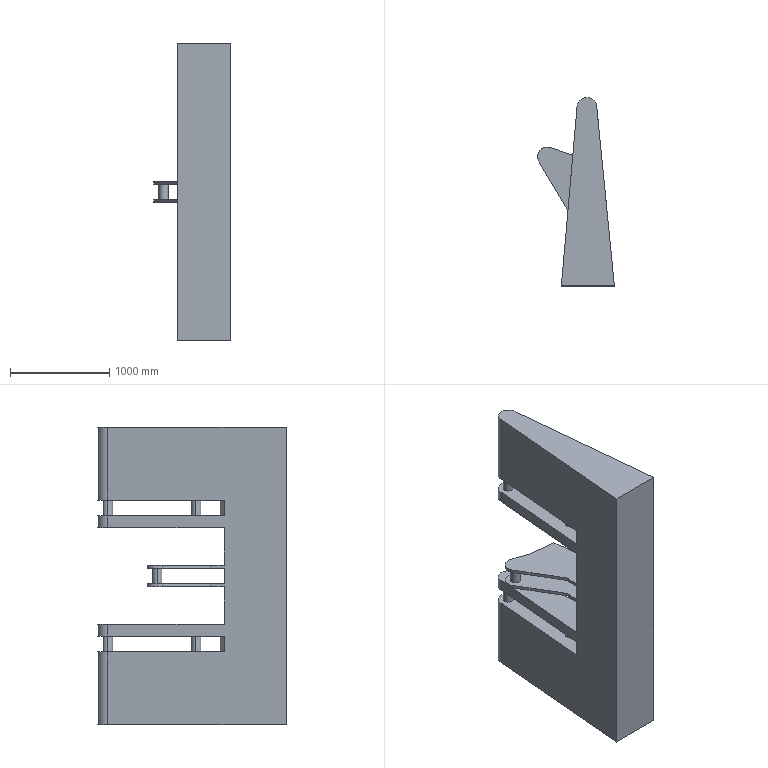Part | SolidWorks | features ICE 8, MirrorPattern 4, Extrusion 1 | 1 solid | 43 faces | box 773.621 x 1900 x 3000 mm | volume 1564577598 mm3 | plane 26 | cylinder 17 | commonest cylinder face diameters 100 x10 200 x7
STEP:
#1=CARTESIAN_POINT('',(534.418,439.01,-2105.5));
#2=VERTEX_POINT('',#1);
#3=CARTESIAN_POINT('',(434.418,439.01,-2105.5));
#4=VERTEX_POINT('',#3);
#5=CARTESIAN_POINT('',(484.418,439.01,-2105.5));
#6=DIRECTION('',(0.,0.,1.));
#7=DIRECTION('',(0.,1.,0.));
#8=AXIS2_PLACEMENT_3D('',#5,#6,#7);
#9=CIRCLE('',#8,50.);
#10=EDGE_CURVE('',#2,#4,#9,.T.);
#11=ORIENTED_EDGE('',*,*,#10,.F.);
#12=CARTESIAN_POINT('',(534.418,439.01,-2265.5));
#13=VERTEX_POINT('',#12);
#14=CARTESIAN_POINT('',(534.418,439.01,-873.079));
#15=DIRECTION('',(0.,0.,-1.));
#16=VECTOR('',#15,1000.);
#17=LINE('',#14,#16);
#18=EDGE_CURVE('',#2,#13,#17,.T.);
#19=ORIENTED_EDGE('',*,*,#18,.T.);
#20=CARTESIAN_POINT('',(434.418,439.01,-2265.5));
#21=VERTEX_POINT('',#20);
#22=CARTESIAN_POINT('',(484.418,439.01,-2265.5));
#23=DIRECTION('',(0.,0.,-1.));
#24=DIRECTION('',(1.,0.,0.));
#25=AXIS2_PLACEMENT_3D('',#22,#23,#24);
#26=CIRCLE('',#25,50.);
#27=EDGE_CURVE('',#21,#13,#26,.T.);
#28=ORIENTED_EDGE('',*,*,#27,.F.);
#29=CARTESIAN_POINT('',(434.418,439.01,-873.079));
#30=DIRECTION('',(0.,0.,-1.));
#31=VECTOR('',#30,1000.);
#32=LINE('',#29,#31);
#33=EDGE_CURVE('',#4,#21,#32,.T.);
#34=ORIENTED_EDGE('',*,*,#33,.F.);
#35=EDGE_LOOP('',(#11,#19,#28,#34));
#36=FACE_OUTER_BOUND('',#35,.T.);
#37=CARTESIAN_POINT('',(484.418,439.01,-873.079));
#38=DIRECTION('',(0.,0.,-1.));
#39=DIRECTION('',(-1.,0.,0.));
#40=AXIS2_PLACEMENT_3D('',#37,#38,#39);
#41=CYLINDRICAL_SURFACE('',#40,50.);
#42=ADVANCED_FACE('',(#36),#41,.T.);
#43=CARTESIAN_POINT('',(434.418,439.01,-894.5));
#44=VERTEX_POINT('',#43);
#45=CARTESIAN_POINT('',(534.418,439.01,-894.5));
#46=VERTEX_POINT('',#45);
#47=CARTESIAN_POINT('',(484.418,439.01,-894.5));
#48=DIRECTION('',(0.,0.,-1.));
#49=DIRECTION('',(0.,1.,0.));
#50=AXIS2_PLACEMENT_3D('',#47,#48,#49);
#51=CIRCLE('',#50,50.);
#52=EDGE_CURVE('',#44,#46,#51,.T.);
#53=ORIENTED_EDGE('',*,*,#52,.F.);
#54=CARTESIAN_POINT('',(434.418,439.01,-734.5));
#55=VERTEX_POINT('',#54);
#56=CARTESIAN_POINT('',(434.418,439.01,-1155.921));
#57=DIRECTION('',(0.,0.,1.));
#58=VECTOR('',#57,1000.);
#59=LINE('',#56,#58);
#60=EDGE_CURVE('',#44,#55,#59,.T.);
#61=ORIENTED_EDGE('',*,*,#60,.T.);
#62=CARTESIAN_POINT('',(534.418,439.01,-734.5));
#63=VERTEX_POINT('',#62);
#64=CARTESIAN_POINT('',(484.418,439.01,-734.5));
#65=DIRECTION('',(0.,0.,1.));
#66=DIRECTION('',(1.,0.,0.));
#67=AXIS2_PLACEMENT_3D('',#64,#65,#66);
#68=CIRCLE('',#67,50.);
#69=EDGE_CURVE('',#63,#55,#68,.T.);
#70=ORIENTED_EDGE('',*,*,#69,.F.);
#71=CARTESIAN_POINT('',(534.418,439.01,-1155.921));
#72=DIRECTION('',(0.,0.,1.));
#73=VECTOR('',#72,1000.);
#74=LINE('',#71,#73);
#75=EDGE_CURVE('',#46,#63,#74,.T.);
#76=ORIENTED_EDGE('',*,*,#75,.F.);
#77=EDGE_LOOP('',(#53,#61,#70,#76));
#78=FACE_OUTER_BOUND('',#77,.T.);
#79=CARTESIAN_POINT('',(484.418,439.01,-1155.921));
#80=DIRECTION('',(0.,0.,1.));
#81=DIRECTION('',(1.,0.,0.));
#82=AXIS2_PLACEMENT_3D('',#79,#80,#81);
#83=CYLINDRICAL_SURFACE('',#82,50.);
#84=ADVANCED_FACE('',(#78),#83,.T.);
#85=CARTESIAN_POINT('',(137.752,831.385,-1580.));
#86=VERTEX_POINT('',#85);
#87=CARTESIAN_POINT('',(37.752,831.385,-1580.));
#88=VERTEX_POINT('',#87);
#89=CARTESIAN_POINT('',(87.752,831.385,-1580.));
#90=DIRECTION('',(0.,0.,1.));
#91=DIRECTION('',(1.,0.,0.));
#92=AXIS2_PLACEMENT_3D('',#89,#90,#91);
#93=CIRCLE('',#92,50.);
#94=EDGE_CURVE('',#86,#88,#93,.T.);
#95=ORIENTED_EDGE('',*,*,#94,.T.);
#96=CARTESIAN_POINT('',(37.752,831.385,-1420.));
#97=VERTEX_POINT('',#96);
#98=CARTESIAN_POINT('',(37.752,831.385,-1751.421));
#99=DIRECTION('',(0.,0.,1.));
#100=VECTOR('',#99,1000.);
#101=LINE('',#98,#100);
#102=EDGE_CURVE('',#88,#97,#101,.T.);
#103=ORIENTED_EDGE('',*,*,#102,.T.);
#104=CARTESIAN_POINT('',(137.752,831.385,-1420.));
#105=VERTEX_POINT('',#104);
#106=CARTESIAN_POINT('',(87.752,831.385,-1420.));
#107=DIRECTION('',(0.,0.,-1.));
#108=DIRECTION('',(1.,0.,0.));
#109=AXIS2_PLACEMENT_3D('',#106,#107,#108);
#110=CIRCLE('',#109,50.);
#111=EDGE_CURVE('',#97,#105,#110,.T.);
#112=ORIENTED_EDGE('',*,*,#111,.T.);
#113=CARTESIAN_POINT('',(137.752,831.385,-1751.421));
#114=DIRECTION('',(0.,0.,1.));
#115=VECTOR('',#114,1000.);
#116=LINE('',#113,#115);
#117=EDGE_CURVE('',#86,#105,#116,.T.);
#118=ORIENTED_EDGE('',*,*,#117,.F.);
#119=EDGE_LOOP('',(#95,#103,#112,#118));
#120=FACE_OUTER_BOUND('',#119,.T.);
#121=CARTESIAN_POINT('',(87.752,831.385,-1751.421));
#122=DIRECTION('',(0.,0.,1.));
#123=DIRECTION('',(1.,0.,0.));
#124=AXIS2_PLACEMENT_3D('',#121,#122,#123);
#125=CYLINDRICAL_SURFACE('',#124,50.);
#126=ADVANCED_FACE('',(#120),#125,.T.);
#127=CARTESIAN_POINT('',(434.418,1329.01,-894.5));
#128=VERTEX_POINT('',#127);
#129=CARTESIAN_POINT('',(534.418,1329.01,-894.5));
#130=VERTEX_POINT('',#129);
#131=CARTESIAN_POINT('',(484.418,1329.01,-894.5));
#132=DIRECTION('',(0.,0.,-1.));
#133=DIRECTION('',(0.,1.,0.));
#134=AXIS2_PLACEMENT_3D('',#131,#132,#133);
#135=CIRCLE('',#134,50.);
#136=EDGE_CURVE('',#128,#130,#135,.T.);
#137=ORIENTED_EDGE('',*,*,#136,.F.);
#138=CARTESIAN_POINT('',(434.418,1329.01,-734.5));
#139=VERTEX_POINT('',#138);
#140=CARTESIAN_POINT('',(434.418,1329.01,-3000.));
#141=DIRECTION('',(0.,0.,1.));
#142=VECTOR('',#141,1000.);
#143=LINE('',#140,#142);
#144=EDGE_CURVE('',#128,#139,#143,.T.);
#145=ORIENTED_EDGE('',*,*,#144,.T.);
#146=CARTESIAN_POINT('',(534.418,1329.01,-734.5));
#147=VERTEX_POINT('',#146);
#148=CARTESIAN_POINT('',(484.418,1329.01,-734.5));
#149=DIRECTION('',(0.,0.,1.));
#150=DIRECTION('',(1.,0.,0.));
#151=AXIS2_PLACEMENT_3D('',#148,#149,#150);
#152=CIRCLE('',#151,50.);
#153=EDGE_CURVE('',#147,#139,#152,.T.);
#154=ORIENTED_EDGE('',*,*,#153,.F.);
#155=CARTESIAN_POINT('',(534.418,1329.01,-3000.));
#156=DIRECTION('',(0.,0.,1.));
#157=VECTOR('',#156,1000.);
#158=LINE('',#155,#157);
#159=EDGE_CURVE('',#130,#147,#158,.T.);
#160=ORIENTED_EDGE('',*,*,#159,.F.);
#161=EDGE_LOOP('',(#137,#145,#154,#160));
#162=FACE_OUTER_BOUND('',#161,.T.);
#163=CARTESIAN_POINT('',(484.418,1329.01,-3000.));
#164=DIRECTION('',(0.,0.,1.));
#165=DIRECTION('',(1.,0.,0.));
#166=AXIS2_PLACEMENT_3D('',#163,#164,#165);
#167=CYLINDRICAL_SURFACE('',#166,50.);
#168=ADVANCED_FACE('',(#162),#167,.T.);
#169=CARTESIAN_POINT('',(534.418,1329.01,-2265.5));
#170=VERTEX_POINT('',#169);
#171=CARTESIAN_POINT('',(434.418,1329.01,-2265.5));
#172=VERTEX_POINT('',#171);
#173=CARTESIAN_POINT('',(484.418,1329.01,-2265.5));
#174=DIRECTION('',(0.,0.,1.));
#175=DIRECTION('',(1.,0.,0.));
#176=AXIS2_PLACEMENT_3D('',#173,#174,#175);
#177=CIRCLE('',#176,50.);
#178=EDGE_CURVE('',#170,#172,#177,.T.);
#179=ORIENTED_EDGE('',*,*,#178,.T.);
#180=CARTESIAN_POINT('',(434.418,1329.01,-2105.5));
#181=VERTEX_POINT('',#180);
#182=CARTESIAN_POINT('',(434.418,1329.01,-3000.));
#183=DIRECTION('',(0.,0.,1.));
#184=VECTOR('',#183,1000.);
#185=LINE('',#182,#184);
#186=EDGE_CURVE('',#172,#181,#185,.T.);
#187=ORIENTED_EDGE('',*,*,#186,.T.);
#188=CARTESIAN_POINT('',(534.418,1329.01,-2105.5));
#189=VERTEX_POINT('',#188);
#190=CARTESIAN_POINT('',(484.418,1329.01,-2105.5));
#191=DIRECTION('',(0.,0.,-1.));
#192=DIRECTION('',(0.,1.,0.));
#193=AXIS2_PLACEMENT_3D('',#190,#191,#192);
#194=CIRCLE('',#193,50.);
#195=EDGE_CURVE('',#181,#189,#194,.T.);
#196=ORIENTED_EDGE('',*,*,#195,.T.);
#197=CARTESIAN_POINT('',(534.418,1329.01,-3000.));
#198=DIRECTION('',(0.,0.,1.));
#199=VECTOR('',#198,1000.);
#200=LINE('',#197,#199);
#201=EDGE_CURVE('',#170,#189,#200,.T.);
#202=ORIENTED_EDGE('',*,*,#201,.F.);
#203=EDGE_LOOP('',(#179,#187,#196,#202));
#204=FACE_OUTER_BOUND('',#203,.T.);
#205=CARTESIAN_POINT('',(484.418,1329.01,-3000.));
#206=DIRECTION('',(0.,0.,1.));
#207=DIRECTION('',(1.,0.,0.));
#208=AXIS2_PLACEMENT_3D('',#205,#206,#207);
#209=CYLINDRICAL_SURFACE('',#208,50.);
#210=ADVANCED_FACE('',(#204),#209,.T.);
#211=CARTESIAN_POINT('',(-12.248,831.385,-1580.));
#212=VERTEX_POINT('',#211);
#213=CARTESIAN_POINT('',(1.855,780.182,-1580.));
#214=VERTEX_POINT('',#213);
#215=CARTESIAN_POINT('',(87.752,831.385,-1580.));
#216=DIRECTION('',(0.,0.,1.));
#217=DIRECTION('',(1.,0.,0.));
#218=AXIS2_PLACEMENT_3D('',#215,#216,#217);
#219=CIRCLE('',#218,100.);
#220=EDGE_CURVE('',#212,#214,#219,.T.);
#221=ORIENTED_EDGE('',*,*,#220,.F.);
#222=CARTESIAN_POINT('',(-12.248,831.385,-1610.));
#223=VERTEX_POINT('',#222);
#224=CARTESIAN_POINT('',(-12.248,831.385,-1580.));
#225=DIRECTION('',(0.,0.,-1.));
#226=VECTOR('',#225,1000.);
#227=LINE('',#224,#226);
#228=EDGE_CURVE('',#212,#223,#227,.T.);
#229=ORIENTED_EDGE('',*,*,#228,.T.);
#230=CARTESIAN_POINT('',(1.855,780.182,-1610.));
#231=VERTEX_POINT('',#230);
#232=CARTESIAN_POINT('',(87.752,831.385,-1610.));
#233=DIRECTION('',(0.,0.,1.));
#234=DIRECTION('',(1.,0.,0.));
#235=AXIS2_PLACEMENT_3D('',#232,#233,#234);
#236=CIRCLE('',#235,100.);
#237=EDGE_CURVE('',#223,#231,#236,.T.);
#238=ORIENTED_EDGE('',*,*,#237,.T.);
#239=CARTESIAN_POINT('',(1.855,780.182,-1580.));
#240=DIRECTION('',(0.,0.,-1.));
#241=VECTOR('',#240,1000.);
#242=LINE('',#239,#241);
#243=EDGE_CURVE('',#214,#231,#242,.T.);
#244=ORIENTED_EDGE('',*,*,#243,.F.);
#245=EDGE_LOOP('',(#221,#229,#238,#244));
#246=FACE_OUTER_BOUND('',#245,.T.);
#247=CARTESIAN_POINT('',(87.752,831.385,-1580.));
#248=DIRECTION('',(0.,0.,-1.));
#249=DIRECTION('',(-1.,0.,0.));
#250=AXIS2_PLACEMENT_3D('',#247,#248,#249);
#251=CYLINDRICAL_SURFACE('',#250,100.);
#252=ADVANCED_FACE('',(#246),#251,.T.);
#253=CARTESIAN_POINT('',(342.529,850.219,-1390.));
#254=VERTEX_POINT('',#253);
#255=CARTESIAN_POINT('',(633.994,824.719,-1390.));
#256=VERTEX_POINT('',#255);
#257=CARTESIAN_POINT('',(76.421,873.5,-1390.));
#258=DIRECTION('',(0.9962,-0.08716,0.));
#259=VECTOR('',#258,1000.);
#260=LINE('',#257,#259);
#261=EDGE_CURVE('',#254,#256,#260,.T.);
#262=ORIENTED_EDGE('',*,*,#261,.F.);
#263=CARTESIAN_POINT('',(120.005,926.041,-1390.));
#264=VERTEX_POINT('',#263);
#265=CARTESIAN_POINT('',(295.197,866.347,-1390.));
#266=DIRECTION('',(0.9466,-0.3225,0.));
#267=VECTOR('',#266,1000.);
#268=LINE('',#265,#267);
#269=EDGE_CURVE('',#264,#254,#268,.T.);
#270=ORIENTED_EDGE('',*,*,#269,.F.);
#271=CARTESIAN_POINT('',(1.855,780.182,-1390.));
#272=VERTEX_POINT('',#271);
#273=CARTESIAN_POINT('',(87.752,831.385,-1390.));
#274=DIRECTION('',(0.,0.,1.));
#275=DIRECTION('',(1.,0.,0.));
#276=AXIS2_PLACEMENT_3D('',#273,#274,#275);
#277=CIRCLE('',#276,100.);
#278=EDGE_CURVE('',#264,#272,#277,.T.);
#279=ORIENTED_EDGE('',*,*,#278,.T.);
#280=CARTESIAN_POINT('',(293.585,290.784,-1390.));
#281=VERTEX_POINT('',#280);
#282=CARTESIAN_POINT('',(344.506,205.36,-1390.));
#283=DIRECTION('',(0.512,-0.859,0.));
#284=VECTOR('',#283,1000.);
#285=LINE('',#282,#284);
#286=EDGE_CURVE('',#272,#281,#285,.T.);
#287=ORIENTED_EDGE('',*,*,#286,.T.);
#288=CARTESIAN_POINT('',(281.586,153.631,-1390.));
#289=VERTEX_POINT('',#288);
#290=CARTESIAN_POINT('',(266.108,-23.281,-1390.));
#291=DIRECTION('',(-0.08716,-0.9962,0.));
#292=VECTOR('',#291,1000.);
#293=LINE('',#290,#292);
#294=EDGE_CURVE('',#281,#289,#293,.T.);
#295=ORIENTED_EDGE('',*,*,#294,.T.);
#296=CARTESIAN_POINT('',(703.597,116.71,-1390.));
#297=VERTEX_POINT('',#296);
#298=CARTESIAN_POINT('',(811.961,107.229,-1390.));
#299=DIRECTION('',(-0.9962,0.08716,0.));
#300=VECTOR('',#299,1000.);
#301=LINE('',#298,#300);
#302=EDGE_CURVE('',#297,#289,#301,.T.);
#303=ORIENTED_EDGE('',*,*,#302,.F.);
#304=CARTESIAN_POINT('',(708.226,69.625,-1390.));
#305=DIRECTION('',(0.09784,-0.9952,0.));
#306=VECTOR('',#305,1000.);
#307=LINE('',#304,#306);
#308=EDGE_CURVE('',#256,#297,#307,.T.);
#309=ORIENTED_EDGE('',*,*,#308,.F.);
#310=EDGE_LOOP('',(#262,#270,#279,#287,#295,#303,#309));
#311=FACE_OUTER_BOUND('',#310,.T.);
#312=CARTESIAN_POINT('',(0.,0.,-1390.));
#313=DIRECTION('',(0.,0.,1.));
#314=DIRECTION('',(1.,0.,0.));
#315=AXIS2_PLACEMENT_3D('',#312,#313,#314);
#316=PLANE('',#315);
#317=ADVANCED_FACE('',(#311),#316,.T.);
#318=CARTESIAN_POINT('',(633.994,824.719,-1610.));
#319=VERTEX_POINT('',#318);
#320=CARTESIAN_POINT('',(342.529,850.219,-1610.));
#321=VERTEX_POINT('',#320);
#322=CARTESIAN_POINT('',(76.421,873.5,-1610.));
#323=DIRECTION('',(-0.9962,0.08716,0.));
#324=VECTOR('',#323,1000.);
#325=LINE('',#322,#324);
#326=EDGE_CURVE('',#319,#321,#325,.T.);
#327=ORIENTED_EDGE('',*,*,#326,.F.);
#328=CARTESIAN_POINT('',(703.597,116.71,-1610.));
#329=VERTEX_POINT('',#328);
#330=CARTESIAN_POINT('',(708.226,69.625,-1610.));
#331=DIRECTION('',(0.09784,-0.9952,0.));
#332=VECTOR('',#331,1000.);
#333=LINE('',#330,#332);
#334=EDGE_CURVE('',#319,#329,#333,.T.);
#335=ORIENTED_EDGE('',*,*,#334,.T.);
#336=CARTESIAN_POINT('',(281.586,153.631,-1610.));
#337=VERTEX_POINT('',#336);
#338=CARTESIAN_POINT('',(811.961,107.229,-1610.));
#339=DIRECTION('',(-0.9962,0.08716,0.));
#340=VECTOR('',#339,1000.);
#341=LINE('',#338,#340);
#342=EDGE_CURVE('',#329,#337,#341,.T.);
#343=ORIENTED_EDGE('',*,*,#342,.T.);
#344=CARTESIAN_POINT('',(293.585,290.784,-1610.));
#345=VERTEX_POINT('',#344);
#346=CARTESIAN_POINT('',(266.108,-23.281,-1610.));
#347=DIRECTION('',(-0.08716,-0.9962,0.));
#348=VECTOR('',#347,1000.);
#349=LINE('',#346,#348);
#350=EDGE_CURVE('',#345,#337,#349,.T.);
#351=ORIENTED_EDGE('',*,*,#350,.F.);
#352=CARTESIAN_POINT('',(344.506,205.36,-1610.));
#353=DIRECTION('',(0.512,-0.859,0.));
#354=VECTOR('',#353,1000.);
#355=LINE('',#352,#354);
#356=EDGE_CURVE('',#231,#345,#355,.T.);
#357=ORIENTED_EDGE('',*,*,#356,.F.);
#358=ORIENTED_EDGE('',*,*,#237,.F.);
#359=CARTESIAN_POINT('',(120.005,926.041,-1610.));
#360=VERTEX_POINT('',#359);
#361=CARTESIAN_POINT('',(87.752,831.385,-1610.));
#362=DIRECTION('',(0.,0.,1.));
#363=DIRECTION('',(1.,0.,0.));
#364=AXIS2_PLACEMENT_3D('',#361,#362,#363);
#365=CIRCLE('',#364,100.);
#366=EDGE_CURVE('',#360,#223,#365,.T.);
#367=ORIENTED_EDGE('',*,*,#366,.F.);
#368=CARTESIAN_POINT('',(295.197,866.347,-1610.));
#369=DIRECTION('',(0.9466,-0.3225,0.));
#370=VECTOR('',#369,1000.);
#371=LINE('',#368,#370);
#372=EDGE_CURVE('',#360,#321,#371,.T.);
#373=ORIENTED_EDGE('',*,*,#372,.T.);
#374=EDGE_LOOP('',(#327,#335,#343,#351,#357,#358,#367,#373));
#375=FACE_OUTER_BOUND('',#374,.T.);
#376=CARTESIAN_POINT('',(0.,0.,-1610.));
#377=DIRECTION('',(0.,0.,-1.));
#378=DIRECTION('',(1.,0.,0.));
#379=AXIS2_PLACEMENT_3D('',#376,#377,#378);
#380=PLANE('',#379);
#381=ADVANCED_FACE('',(#375),#380,.T.);
#382=CARTESIAN_POINT('',(384.418,1329.01,-2105.5));
#383=VERTEX_POINT('',#382);
#384=CARTESIAN_POINT('',(384.418,1329.01,-1985.5));
#385=VERTEX_POINT('',#384);
#386=CARTESIAN_POINT('',(384.418,1329.01,-3000.));
#387=DIRECTION('',(0.,0.,1.));
#388=VECTOR('',#387,1000.);
#389=LINE('',#386,#388);
#390=EDGE_CURVE('',#383,#385,#389,.T.);
#391=ORIENTED_EDGE('',*,*,#390,.T.);
#392=CARTESIAN_POINT('',(584.418,1329.01,-1985.5));
#393=VERTEX_POINT('',#392);
#394=CARTESIAN_POINT('',(484.418,1329.01,-1985.5));
#395=DIRECTION('',(0.,0.,-1.));
#396=DIRECTION('',(0.,-1.,0.));
#397=AXIS2_PLACEMENT_3D('',#394,#395,#396);
#398=CIRCLE('',#397,100.);
#399=EDGE_CURVE('',#385,#393,#398,.T.);
#400=ORIENTED_EDGE('',*,*,#399,.T.);
#401=CARTESIAN_POINT('',(584.418,1329.01,-2105.5));
#402=VERTEX_POINT('',#401);
#403=CARTESIAN_POINT('',(584.418,1329.01,-3000.));
#404=DIRECTION('',(0.,0.,1.));
#405=VECTOR('',#404,1000.);
#406=LINE('',#403,#405);
#407=EDGE_CURVE('',#402,#393,#406,.T.);
#408=ORIENTED_EDGE('',*,*,#407,.F.);
#409=CARTESIAN_POINT('',(484.418,1329.01,-2105.5));
#410=DIRECTION('',(0.,0.,1.));
#411=DIRECTION('',(0.,1.,0.));
#412=AXIS2_PLACEMENT_3D('',#409,#410,#411);
#413=CIRCLE('',#412,100.);
#414=EDGE_CURVE('',#402,#383,#413,.T.);
#415=ORIENTED_EDGE('',*,*,#414,.T.);
#416=EDGE_LOOP('',(#391,#400,#408,#415));
#417=FACE_OUTER_BOUND('',#416,.T.);
#418=CARTESIAN_POINT('',(484.418,1329.01,-3000.));
#419=DIRECTION('',(0.,0.,1.));
#420=DIRECTION('',(1.,0.,0.));
#421=AXIS2_PLACEMENT_3D('',#418,#419,#420);
#422=CYLINDRICAL_SURFACE('',#421,100.);
#423=ADVANCED_FACE('',(#417),#422,.T.);
#424=CARTESIAN_POINT('',(281.586,153.631,-1420.));
#425=VERTEX_POINT('',#424);
#426=CARTESIAN_POINT('',(293.585,290.784,-1420.));
#427=VERTEX_POINT('',#426);
#428=CARTESIAN_POINT('',(342.529,850.219,-1420.));
#429=DIRECTION('',(0.08716,0.9962,0.));
#430=VECTOR('',#429,1000.);
#431=LINE('',#428,#430);
#432=EDGE_CURVE('',#425,#427,#431,.T.);
#433=ORIENTED_EDGE('',*,*,#432,.F.);
#434=CARTESIAN_POINT('',(281.586,153.631,-1580.));
#435=VERTEX_POINT('',#434);
#436=CARTESIAN_POINT('',(281.586,153.631,-1580.));
#437=DIRECTION('',(0.,0.,1.));
#438=VECTOR('',#437,1000.);
#439=LINE('',#436,#438);
#440=EDGE_CURVE('',#435,#425,#439,.T.);
#441=ORIENTED_EDGE('',*,*,#440,.F.);
#442=CARTESIAN_POINT('',(293.585,290.784,-1580.));
#443=VERTEX_POINT('',#442);
#444=CARTESIAN_POINT('',(342.529,850.219,-1580.));
#445=DIRECTION('',(-0.08716,-0.9962,0.));
#446=VECTOR('',#445,1000.);
#447=LINE('',#444,#446);
#448=EDGE_CURVE('',#443,#435,#447,.T.);
#449=ORIENTED_EDGE('',*,*,#448,.F.);
#450=CARTESIAN_POINT('',(293.585,290.784,-1580.));
#451=DIRECTION('',(0.,0.,-1.));
#452=VECTOR('',#451,1000.);
#453=LINE('',#450,#452);
#454=EDGE_CURVE('',#443,#345,#453,.T.);
#455=ORIENTED_EDGE('',*,*,#454,.T.);
#456=ORIENTED_EDGE('',*,*,#350,.T.);
#457=CARTESIAN_POINT('',(281.586,153.631,-1985.5));
#458=VERTEX_POINT('',#457);
#459=CARTESIAN_POINT('',(281.586,153.631,-3000.));
#460=DIRECTION('',(0.,0.,-1.));
#461=VECTOR('',#460,1000.);
#462=LINE('',#459,#461);
#463=EDGE_CURVE('',#337,#458,#462,.T.);
#464=ORIENTED_EDGE('',*,*,#463,.T.);
#465=CARTESIAN_POINT('',(266.108,-23.281,-1985.5));
#466=DIRECTION('',(0.08716,0.9962,0.));
#467=VECTOR('',#466,1000.);
#468=LINE('',#465,#467);
#469=EDGE_CURVE('',#458,#385,#468,.T.);
#470=ORIENTED_EDGE('',*,*,#469,.T.);
#471=ORIENTED_EDGE('',*,*,#390,.F.);
#472=CARTESIAN_POINT('',(281.586,153.631,-2105.5));
#473=VERTEX_POINT('',#472);
#474=CARTESIAN_POINT('',(266.108,-23.281,-2105.5));
#475=DIRECTION('',(-0.08716,-0.9962,0.));
#476=VECTOR('',#475,1000.);
#477=LINE('',#474,#476);
#478=EDGE_CURVE('',#383,#473,#477,.T.);
#479=ORIENTED_EDGE('',*,*,#478,.T.);
#480=CARTESIAN_POINT('',(281.586,153.631,-2265.5));
#481=VERTEX_POINT('',#480);
#482=CARTESIAN_POINT('',(281.586,153.631,-3000.));
#483=DIRECTION('',(0.,0.,-1.));
#484=VECTOR('',#483,1000.);
#485=LINE('',#482,#484);
#486=EDGE_CURVE('',#473,#481,#485,.T.);
#487=ORIENTED_EDGE('',*,*,#486,.T.);
#488=CARTESIAN_POINT('',(384.418,1329.01,-2265.5));
#489=VERTEX_POINT('',#488);
#490=CARTESIAN_POINT('',(266.108,-23.281,-2265.5));
#491=DIRECTION('',(0.08716,0.9962,0.));
#492=VECTOR('',#491,1000.);
#493=LINE('',#490,#492);
#494=EDGE_CURVE('',#481,#489,#493,.T.);
#495=ORIENTED_EDGE('',*,*,#494,.T.);
#496=CARTESIAN_POINT('',(384.418,1329.01,-3000.));
#497=VERTEX_POINT('',#496);
#498=CARTESIAN_POINT('',(384.418,1329.01,-3000.));
#499=DIRECTION('',(0.,0.,1.));
#500=VECTOR('',#499,1000.);
#501=LINE('',#498,#500);
#502=EDGE_CURVE('',#497,#489,#501,.T.);
#503=ORIENTED_EDGE('',*,*,#502,.F.);
#504=CARTESIAN_POINT('',(226.938,-470.99,-3000.));
#505=VERTEX_POINT('',#504);
#506=CARTESIAN_POINT('',(266.108,-23.281,-3000.));
#507=DIRECTION('',(-0.08716,-0.9962,0.));
#508=VECTOR('',#507,1000.);
#509=LINE('',#506,#508);
#510=EDGE_CURVE('',#497,#505,#509,.T.);
#511=ORIENTED_EDGE('',*,*,#510,.T.);
#512=CARTESIAN_POINT('',(226.938,-470.99,0.));
#513=VERTEX_POINT('',#512);
#514=CARTESIAN_POINT('',(226.938,-470.99,-3000.));
#515=DIRECTION('',(0.,0.,1.));
#516=VECTOR('',#515,1000.);
#517=LINE('',#514,#516);
#518=EDGE_CURVE('',#505,#513,#517,.T.);
#519=ORIENTED_EDGE('',*,*,#518,.T.);
#520=CARTESIAN_POINT('',(384.418,1329.01,0.));
#521=VERTEX_POINT('',#520);
#522=CARTESIAN_POINT('',(266.108,-23.281,0.));
#523=DIRECTION('',(-0.08716,-0.9962,0.));
#524=VECTOR('',#523,1000.);
#525=LINE('',#522,#524);
#526=EDGE_CURVE('',#521,#513,#525,.T.);
#527=ORIENTED_EDGE('',*,*,#526,.F.);
#528=CARTESIAN_POINT('',(384.418,1329.01,-734.5));
#529=VERTEX_POINT('',#528);
#530=CARTESIAN_POINT('',(384.418,1329.01,-3000.));
#531=DIRECTION('',(0.,0.,1.));
#532=VECTOR('',#531,1000.);
#533=LINE('',#530,#532);
#534=EDGE_CURVE('',#529,#521,#533,.T.);
#535=ORIENTED_EDGE('',*,*,#534,.F.);
#536=CARTESIAN_POINT('',(281.586,153.631,-734.5));
#537=VERTEX_POINT('',#536);
#538=CARTESIAN_POINT('',(266.108,-23.281,-734.5));
#539=DIRECTION('',(0.08716,0.9962,0.));
#540=VECTOR('',#539,1000.);
#541=LINE('',#538,#540);
#542=EDGE_CURVE('',#537,#529,#541,.T.);
#543=ORIENTED_EDGE('',*,*,#542,.F.);
#544=CARTESIAN_POINT('',(281.586,153.631,-894.5));
#545=VERTEX_POINT('',#544);
#546=CARTESIAN_POINT('',(281.586,153.631,-3000.));
#547=DIRECTION('',(0.,0.,1.));
#548=VECTOR('',#547,1000.);
#549=LINE('',#546,#548);
#550=EDGE_CURVE('',#545,#537,#549,.T.);
#551=ORIENTED_EDGE('',*,*,#550,.F.);
#552=CARTESIAN_POINT('',(384.418,1329.01,-894.5));
#553=VERTEX_POINT('',#552);
#554=CARTESIAN_POINT('',(266.108,-23.281,-894.5));
#555=DIRECTION('',(-0.08716,-0.9962,0.));
#556=VECTOR('',#555,1000.);
#557=LINE('',#554,#556);
#558=EDGE_CURVE('',#553,#545,#557,.T.);
#559=ORIENTED_EDGE('',*,*,#558,.F.);
#560=CARTESIAN_POINT('',(384.418,1329.01,-1014.5));
#561=VERTEX_POINT('',#560);
#562=CARTESIAN_POINT('',(384.418,1329.01,-3000.));
#563=DIRECTION('',(0.,0.,1.));
#564=VECTOR('',#563,1000.);
#565=LINE('',#562,#564);
#566=EDGE_CURVE('',#561,#553,#565,.T.);
#567=ORIENTED_EDGE('',*,*,#566,.F.);
#568=CARTESIAN_POINT('',(281.586,153.631,-1014.5));
#569=VERTEX_POINT('',#568);
#570=CARTESIAN_POINT('',(266.108,-23.281,-1014.5));
#571=DIRECTION('',(0.08716,0.9962,0.));
#572=VECTOR('',#571,1000.);
#573=LINE('',#570,#572);
#574=EDGE_CURVE('',#569,#561,#573,.T.);
#575=ORIENTED_EDGE('',*,*,#574,.F.);
#576=CARTESIAN_POINT('',(281.586,153.631,-3000.));
#577=DIRECTION('',(0.,0.,1.));
#578=VECTOR('',#577,1000.);
#579=LINE('',#576,#578);
#580=EDGE_CURVE('',#289,#569,#579,.T.);
#581=ORIENTED_EDGE('',*,*,#580,.F.);
#582=ORIENTED_EDGE('',*,*,#294,.F.);
#583=CARTESIAN_POINT('',(293.585,290.784,-1420.));
#584=DIRECTION('',(0.,0.,1.));
#585=VECTOR('',#584,1000.);
#586=LINE('',#583,#585);
#587=EDGE_CURVE('',#427,#281,#586,.T.);
#588=ORIENTED_EDGE('',*,*,#587,.F.);
#589=EDGE_LOOP('',(#433,#441,#449,#455,#456,#464,#470,#471,#479,#487,#495,#503,#511,#519,#527,#535,#543,#551,#559,#567,#575,#581,#582,#588));
#590=FACE_OUTER_BOUND('',#589,.T.);
#591=CARTESIAN_POINT('',(266.108,-23.281,-3000.));
#592=DIRECTION('',(-0.9962,0.08716,0.));
#593=DIRECTION('',(-0.08716,-0.9962,0.));
#594=AXIS2_PLACEMENT_3D('',#591,#592,#593);
#595=PLANE('',#594);
#596=ADVANCED_FACE('',(#590),#595,.T.);
#597=ORIENTED_EDGE('',*,*,#334,.F.);
#598=CARTESIAN_POINT('',(633.994,824.719,-1580.));
#599=VERTEX_POINT('',#598);
#600=CARTESIAN_POINT('',(633.994,824.719,-3000.));
#601=DIRECTION('',(0.,0.,1.));
#602=VECTOR('',#601,1000.);
#603=LINE('',#600,#602);
#604=EDGE_CURVE('',#319,#599,#603,.T.);
#605=ORIENTED_EDGE('',*,*,#604,.T.);
#606=CARTESIAN_POINT('',(703.597,116.71,-1580.));
#607=VERTEX_POINT('',#606);
#608=CARTESIAN_POINT('',(708.226,69.625,-1580.));
#609=DIRECTION('',(0.09784,-0.9952,0.));
#610=VECTOR('',#609,1000.);
#611=LINE('',#608,#610);
#612=EDGE_CURVE('',#599,#607,#611,.T.);
#613=ORIENTED_EDGE('',*,*,#612,.T.);
#614=CARTESIAN_POINT('',(703.597,116.71,-1420.));
#615=VERTEX_POINT('',#614);
#616=CARTESIAN_POINT('',(703.597,116.71,-3000.));
#617=DIRECTION('',(0.,0.,1.));
#618=VECTOR('',#617,1000.);
#619=LINE('',#616,#618);
#620=EDGE_CURVE('',#607,#615,#619,.T.);
#621=ORIENTED_EDGE('',*,*,#620,.T.);
#622=CARTESIAN_POINT('',(633.994,824.719,-1420.));
#623=VERTEX_POINT('',#622);
#624=CARTESIAN_POINT('',(708.226,69.625,-1420.));
#625=DIRECTION('',(-0.09784,0.9952,0.));
#626=VECTOR('',#625,1000.);
#627=LINE('',#624,#626);
#628=EDGE_CURVE('',#615,#623,#627,.T.);
#629=ORIENTED_EDGE('',*,*,#628,.T.);
#630=CARTESIAN_POINT('',(633.994,824.719,-3000.));
#631=DIRECTION('',(0.,0.,1.));
#632=VECTOR('',#631,1000.);
#633=LINE('',#630,#632);
#634=EDGE_CURVE('',#623,#256,#633,.T.);
#635=ORIENTED_EDGE('',*,*,#634,.T.);
#636=ORIENTED_EDGE('',*,*,#308,.T.);
#637=CARTESIAN_POINT('',(703.597,116.71,-1014.5));
#638=VERTEX_POINT('',#637);
#639=CARTESIAN_POINT('',(703.597,116.71,-3000.));
#640=DIRECTION('',(0.,0.,1.));
#641=VECTOR('',#640,1000.);
#642=LINE('',#639,#641);
#643=EDGE_CURVE('',#297,#638,#642,.T.);
#644=ORIENTED_EDGE('',*,*,#643,.T.);
#645=CARTESIAN_POINT('',(584.418,1329.01,-1014.5));
#646=VERTEX_POINT('',#645);
#647=CARTESIAN_POINT('',(708.226,69.625,-1014.5));
#648=DIRECTION('',(-0.09784,0.9952,0.));
#649=VECTOR('',#648,1000.);
#650=LINE('',#647,#649);
#651=EDGE_CURVE('',#638,#646,#650,.T.);
#652=ORIENTED_EDGE('',*,*,#651,.T.);
#653=CARTESIAN_POINT('',(584.418,1329.01,-894.5));
#654=VERTEX_POINT('',#653);
#655=CARTESIAN_POINT('',(584.418,1329.01,-3000.));
#656=DIRECTION('',(0.,0.,1.));
#657=VECTOR('',#656,1000.);
#658=LINE('',#655,#657);
#659=EDGE_CURVE('',#646,#654,#658,.T.);
#660=ORIENTED_EDGE('',*,*,#659,.T.);
#661=CARTESIAN_POINT('',(695.963,194.368,-894.5));
#662=VERTEX_POINT('',#661);
#663=CARTESIAN_POINT('',(708.226,69.625,-894.5));
#664=DIRECTION('',(0.09784,-0.9952,0.));
#665=VECTOR('',#664,1000.);
#666=LINE('',#663,#665);
#667=EDGE_CURVE('',#654,#662,#666,.T.);
#668=ORIENTED_EDGE('',*,*,#667,.T.);
#669=CARTESIAN_POINT('',(695.963,194.368,-734.5));
#670=VERTEX_POINT('',#669);
#671=CARTESIAN_POINT('',(695.963,194.368,-3000.));
#672=DIRECTION('',(0.,0.,1.));
#673=VECTOR('',#672,1000.);
#674=LINE('',#671,#673);
#675=EDGE_CURVE('',#662,#670,#674,.T.);
#676=ORIENTED_EDGE('',*,*,#675,.T.);
#677=CARTESIAN_POINT('',(584.418,1329.01,-734.5));
#678=VERTEX_POINT('',#677);
#679=CARTESIAN_POINT('',(708.226,69.625,-734.5));
#680=DIRECTION('',(-0.09784,0.9952,0.));
#681=VECTOR('',#680,1000.);
#682=LINE('',#679,#681);
#683=EDGE_CURVE('',#670,#678,#682,.T.);
#684=ORIENTED_EDGE('',*,*,#683,.T.);
#685=CARTESIAN_POINT('',(584.418,1329.01,0.));
#686=VERTEX_POINT('',#685);
#687=CARTESIAN_POINT('',(584.418,1329.01,-3000.));
#688=DIRECTION('',(0.,0.,1.));
#689=VECTOR('',#688,1000.);
#690=LINE('',#687,#689);
#691=EDGE_CURVE('',#678,#686,#690,.T.);
#692=ORIENTED_EDGE('',*,*,#691,.T.);
#693=CARTESIAN_POINT('',(761.373,-470.99,0.));
#694=VERTEX_POINT('',#693);
#695=CARTESIAN_POINT('',(708.226,69.625,0.));
#696=DIRECTION('',(0.09784,-0.9952,0.));
#697=VECTOR('',#696,1000.);
#698=LINE('',#695,#697);
#699=EDGE_CURVE('',#686,#694,#698,.T.);
#700=ORIENTED_EDGE('',*,*,#699,.T.);
#701=CARTESIAN_POINT('',(761.373,-470.99,-3000.));
#702=VERTEX_POINT('',#701);
#703=CARTESIAN_POINT('',(761.373,-470.99,-3000.));
#704=DIRECTION('',(0.,0.,1.));
#705=VECTOR('',#704,1000.);
#706=LINE('',#703,#705);
#707=EDGE_CURVE('',#702,#694,#706,.T.);
#708=ORIENTED_EDGE('',*,*,#707,.F.);
#709=CARTESIAN_POINT('',(584.418,1329.01,-3000.));
#710=VERTEX_POINT('',#709);
#711=CARTESIAN_POINT('',(708.226,69.625,-3000.));
#712=DIRECTION('',(0.09784,-0.9952,0.));
#713=VECTOR('',#712,1000.);
#714=LINE('',#711,#713);
#715=EDGE_CURVE('',#710,#702,#714,.T.);
#716=ORIENTED_EDGE('',*,*,#715,.F.);
#717=CARTESIAN_POINT('',(584.418,1329.01,-2265.5));
#718=VERTEX_POINT('',#717);
#719=CARTESIAN_POINT('',(584.418,1329.01,-3000.));
#720=DIRECTION('',(0.,0.,1.));
#721=VECTOR('',#720,1000.);
#722=LINE('',#719,#721);
#723=EDGE_CURVE('',#710,#718,#722,.T.);
#724=ORIENTED_EDGE('',*,*,#723,.T.);
#725=CARTESIAN_POINT('',(695.963,194.368,-2265.5));
#726=VERTEX_POINT('',#725);
#727=CARTESIAN_POINT('',(708.226,69.625,-2265.5));
#728=DIRECTION('',(-0.09784,0.9952,0.));
#729=VECTOR('',#728,1000.);
#730=LINE('',#727,#729);
#731=EDGE_CURVE('',#726,#718,#730,.T.);
#732=ORIENTED_EDGE('',*,*,#731,.F.);
#733=CARTESIAN_POINT('',(695.963,194.368,-2105.5));
#734=VERTEX_POINT('',#733);
#735=CARTESIAN_POINT('',(695.963,194.368,-3000.));
#736=DIRECTION('',(0.,0.,-1.));
#737=VECTOR('',#736,1000.);
#738=LINE('',#735,#737);
#739=EDGE_CURVE('',#734,#726,#738,.T.);
#740=ORIENTED_EDGE('',*,*,#739,.F.);
#741=CARTESIAN_POINT('',(708.226,69.625,-2105.5));
#742=DIRECTION('',(0.09784,-0.9952,0.));
#743=VECTOR('',#742,1000.);
#744=LINE('',#741,#743);
#745=EDGE_CURVE('',#402,#734,#744,.T.);
#746=ORIENTED_EDGE('',*,*,#745,.F.);
#747=ORIENTED_EDGE('',*,*,#407,.T.);
#748=CARTESIAN_POINT('',(703.597,116.71,-1985.5));
#749=VERTEX_POINT('',#748);
#750=CARTESIAN_POINT('',(708.226,69.625,-1985.5));
#751=DIRECTION('',(-0.09784,0.9952,0.));
#752=VECTOR('',#751,1000.);
#753=LINE('',#750,#752);
#754=EDGE_CURVE('',#749,#393,#753,.T.);
#755=ORIENTED_EDGE('',*,*,#754,.F.);
#756=CARTESIAN_POINT('',(703.597,116.71,-3000.));
#757=DIRECTION('',(0.,0.,-1.));
#758=VECTOR('',#757,1000.);
#759=LINE('',#756,#758);
#760=EDGE_CURVE('',#329,#749,#759,.T.);
#761=ORIENTED_EDGE('',*,*,#760,.F.);
#762=EDGE_LOOP('',(#597,#605,#613,#621,#629,#635,#636,#644,#652,#660,#668,#676,#684,#692,#700,#708,#716,#724,#732,#740,#746,#747,#755,#761));
#763=FACE_OUTER_BOUND('',#762,.T.);
#764=CARTESIAN_POINT('',(708.226,69.625,-3000.));
#765=DIRECTION('',(-0.9952,-0.09784,0.));
#766=DIRECTION('',(0.09784,-0.9952,0.));
#767=AXIS2_PLACEMENT_3D('',#764,#765,#766);
#768=PLANE('',#767);
#769=ADVANCED_FACE('',(#763),#768,.F.);
#770=ORIENTED_EDGE('',*,*,#502,.T.);
#771=CARTESIAN_POINT('',(484.418,1329.01,-2265.5));
#772=DIRECTION('',(0.,0.,-1.));
#773=DIRECTION('',(1.,0.,0.));
#774=AXIS2_PLACEMENT_3D('',#771,#772,#773);
#775=CIRCLE('',#774,100.);
#776=EDGE_CURVE('',#489,#718,#775,.T.);
#777=ORIENTED_EDGE('',*,*,#776,.T.);
#778=ORIENTED_EDGE('',*,*,#723,.F.);
#779=CARTESIAN_POINT('',(484.418,1329.01,-3000.));
#780=DIRECTION('',(0.,0.,1.));
#781=DIRECTION('',(1.,0.,0.));
#782=AXIS2_PLACEMENT_3D('',#779,#780,#781);
#783=CIRCLE('',#782,100.);
#784=EDGE_CURVE('',#710,#497,#783,.T.);
#785=ORIENTED_EDGE('',*,*,#784,.T.);
#786=EDGE_LOOP('',(#770,#777,#778,#785));
#787=FACE_OUTER_BOUND('',#786,.T.);
#788=CARTESIAN_POINT('',(484.418,1329.01,-3000.));
#789=DIRECTION('',(0.,0.,1.));
#790=DIRECTION('',(1.,0.,0.));
#791=AXIS2_PLACEMENT_3D('',#788,#789,#790);
#792=CYLINDRICAL_SURFACE('',#791,100.);
#793=ADVANCED_FACE('',(#787),#792,.T.);
#794=CARTESIAN_POINT('',(484.418,1329.01,-1014.5));
#795=DIRECTION('',(0.,0.,-1.));
#796=DIRECTION('',(0.,-1.,0.));
#797=AXIS2_PLACEMENT_3D('',#794,#795,#796);
#798=CIRCLE('',#797,100.);
#799=EDGE_CURVE('',#561,#646,#798,.T.);
#800=ORIENTED_EDGE('',*,*,#799,.F.);
#801=ORIENTED_EDGE('',*,*,#566,.T.);
#802=CARTESIAN_POINT('',(484.418,1329.01,-894.5));
#803=DIRECTION('',(0.,0.,1.));
#804=DIRECTION('',(0.,1.,0.));
#805=AXIS2_PLACEMENT_3D('',#802,#803,#804);
#806=CIRCLE('',#805,100.);
#807=EDGE_CURVE('',#654,#553,#806,.T.);
#808=ORIENTED_EDGE('',*,*,#807,.F.);
#809=ORIENTED_EDGE('',*,*,#659,.F.);
#810=EDGE_LOOP('',(#800,#801,#808,#809));
#811=FACE_OUTER_BOUND('',#810,.T.);
#812=CARTESIAN_POINT('',(484.418,1329.01,-3000.));
#813=DIRECTION('',(0.,0.,1.));
#814=DIRECTION('',(1.,0.,0.));
#815=AXIS2_PLACEMENT_3D('',#812,#813,#814);
#816=CYLINDRICAL_SURFACE('',#815,100.);
#817=ADVANCED_FACE('',(#811),#816,.T.);
#818=CARTESIAN_POINT('',(484.418,1329.01,-734.5));
#819=DIRECTION('',(0.,0.,-1.));
#820=DIRECTION('',(1.,0.,0.));
#821=AXIS2_PLACEMENT_3D('',#818,#819,#820);
#822=CIRCLE('',#821,100.);
#823=EDGE_CURVE('',#529,#678,#822,.T.);
#824=ORIENTED_EDGE('',*,*,#823,.F.);
#825=ORIENTED_EDGE('',*,*,#534,.T.);
#826=CARTESIAN_POINT('',(484.418,1329.01,0.));
#827=DIRECTION('',(0.,0.,1.));
#828=DIRECTION('',(1.,0.,0.));
#829=AXIS2_PLACEMENT_3D('',#826,#827,#828);
#830=CIRCLE('',#829,100.);
#831=EDGE_CURVE('',#686,#521,#830,.T.);
#832=ORIENTED_EDGE('',*,*,#831,.F.);
#833=ORIENTED_EDGE('',*,*,#691,.F.);
#834=EDGE_LOOP('',(#824,#825,#832,#833));
#835=FACE_OUTER_BOUND('',#834,.T.);
#836=CARTESIAN_POINT('',(484.418,1329.01,-3000.));
#837=DIRECTION('',(0.,0.,1.));
#838=DIRECTION('',(1.,0.,0.));
#839=AXIS2_PLACEMENT_3D('',#836,#837,#838);
#840=CYLINDRICAL_SURFACE('',#839,100.);
#841=ADVANCED_FACE('',(#835),#840,.T.);
#842=CARTESIAN_POINT('',(0.,-470.99,0.));
#843=DIRECTION('',(1.,0.,0.));
#844=VECTOR('',#843,1000.);
#845=LINE('',#842,#844);
#846=EDGE_CURVE('',#513,#694,#845,.T.);
#847=ORIENTED_EDGE('',*,*,#846,.F.);
#848=ORIENTED_EDGE('',*,*,#518,.F.);
#849=CARTESIAN_POINT('',(0.,-470.99,-3000.));
#850=DIRECTION('',(1.,0.,0.));
#851=VECTOR('',#850,1000.);
#852=LINE('',#849,#851);
#853=EDGE_CURVE('',#505,#702,#852,.T.);
#854=ORIENTED_EDGE('',*,*,#853,.T.);
#855=ORIENTED_EDGE('',*,*,#707,.T.);
#856=EDGE_LOOP('',(#847,#848,#854,#855));
#857=FACE_OUTER_BOUND('',#856,.T.);
#858=CARTESIAN_POINT('',(0.,-470.99,-3000.));
#859=DIRECTION('',(0.,-1.,0.));
#860=DIRECTION('',(1.,0.,0.));
#861=AXIS2_PLACEMENT_3D('',#858,#859,#860);
#862=PLANE('',#861);
#863=ADVANCED_FACE('',(#857),#862,.T.);
#864=ORIENTED_EDGE('',*,*,#715,.T.);
#865=ORIENTED_EDGE('',*,*,#853,.F.);
#866=ORIENTED_EDGE('',*,*,#510,.F.);
#867=ORIENTED_EDGE('',*,*,#784,.F.);
#868=EDGE_LOOP('',(#864,#865,#866,#867));
#869=FACE_OUTER_BOUND('',#868,.T.);
#870=CARTESIAN_POINT('',(0.,0.,-3000.));
#871=DIRECTION('',(0.,0.,1.));
#872=DIRECTION('',(1.,0.,0.));
#873=AXIS2_PLACEMENT_3D('',#870,#871,#872);
#874=PLANE('',#873);
#875=ADVANCED_FACE('',(#869),#874,.F.);
#876=ORIENTED_EDGE('',*,*,#699,.F.);
#877=ORIENTED_EDGE('',*,*,#831,.T.);
#878=ORIENTED_EDGE('',*,*,#526,.T.);
#879=ORIENTED_EDGE('',*,*,#846,.T.);
#880=EDGE_LOOP('',(#876,#877,#878,#879));
#881=FACE_OUTER_BOUND('',#880,.T.);
#882=CARTESIAN_POINT('',(0.,0.,0.));
#883=DIRECTION('',(0.,0.,1.));
#884=DIRECTION('',(1.,0.,0.));
#885=AXIS2_PLACEMENT_3D('',#882,#883,#884);
#886=PLANE('',#885);
#887=ADVANCED_FACE('',(#881),#886,.T.);
#888=ORIENTED_EDGE('',*,*,#269,.T.);
#889=CARTESIAN_POINT('',(342.529,850.219,-1420.));
#890=VERTEX_POINT('',#889);
#891=CARTESIAN_POINT('',(342.529,850.219,-1420.));
#892=DIRECTION('',(0.,0.,1.));
#893=VECTOR('',#892,1000.);
#894=LINE('',#891,#893);
#895=EDGE_CURVE('',#890,#254,#894,.T.);
#896=ORIENTED_EDGE('',*,*,#895,.F.);
#897=CARTESIAN_POINT('',(120.005,926.041,-1420.));
#898=VERTEX_POINT('',#897);
#899=CARTESIAN_POINT('',(295.197,866.347,-1420.));
#900=DIRECTION('',(0.9466,-0.3225,0.));
#901=VECTOR('',#900,1000.);
#902=LINE('',#899,#901);
#903=EDGE_CURVE('',#898,#890,#902,.T.);
#904=ORIENTED_EDGE('',*,*,#903,.F.);
#905=CARTESIAN_POINT('',(120.005,926.041,-1420.));
#906=DIRECTION('',(0.,0.,1.));
#907=VECTOR('',#906,1000.);
#908=LINE('',#905,#907);
#909=EDGE_CURVE('',#898,#264,#908,.T.);
#910=ORIENTED_EDGE('',*,*,#909,.T.);
#911=EDGE_LOOP('',(#888,#896,#904,#910));
#912=FACE_OUTER_BOUND('',#911,.T.);
#913=CARTESIAN_POINT('',(295.197,866.347,-1420.));
#914=DIRECTION('',(-0.3225,-0.9466,0.));
#915=DIRECTION('',(0.9466,-0.3225,0.));
#916=AXIS2_PLACEMENT_3D('',#913,#914,#915);
#917=PLANE('',#916);
#918=ADVANCED_FACE('',(#912),#917,.F.);
#919=ORIENTED_EDGE('',*,*,#286,.F.);
#920=CARTESIAN_POINT('',(1.855,780.182,-1420.));
#921=VERTEX_POINT('',#920);
#922=CARTESIAN_POINT('',(1.855,780.182,-1420.));
#923=DIRECTION('',(0.,0.,1.));
#924=VECTOR('',#923,1000.);
#925=LINE('',#922,#924);
#926=EDGE_CURVE('',#921,#272,#925,.T.);
#927=ORIENTED_EDGE('',*,*,#926,.F.);
#928=CARTESIAN_POINT('',(344.506,205.36,-1420.));
#929=DIRECTION('',(0.512,-0.859,0.));
#930=VECTOR('',#929,1000.);
#931=LINE('',#928,#930);
#932=EDGE_CURVE('',#921,#427,#931,.T.);
#933=ORIENTED_EDGE('',*,*,#932,.T.);
#934=ORIENTED_EDGE('',*,*,#587,.T.);
#935=EDGE_LOOP('',(#919,#927,#933,#934));
#936=FACE_OUTER_BOUND('',#935,.T.);
#937=CARTESIAN_POINT('',(344.506,205.36,-1420.));
#938=DIRECTION('',(-0.859,-0.512,0.));
#939=DIRECTION('',(0.512,-0.859,0.));
#940=AXIS2_PLACEMENT_3D('',#937,#938,#939);
#941=PLANE('',#940);
#942=ADVANCED_FACE('',(#936),#941,.T.);
#943=ORIENTED_EDGE('',*,*,#278,.F.);
#944=ORIENTED_EDGE('',*,*,#909,.F.);
#945=CARTESIAN_POINT('',(87.752,831.385,-1420.));
#946=DIRECTION('',(0.,0.,1.));
#947=DIRECTION('',(1.,0.,0.));
#948=AXIS2_PLACEMENT_3D('',#945,#946,#947);
#949=CIRCLE('',#948,100.);
#950=EDGE_CURVE('',#898,#921,#949,.T.);
#951=ORIENTED_EDGE('',*,*,#950,.T.);
#952=ORIENTED_EDGE('',*,*,#926,.T.);
#953=EDGE_LOOP('',(#943,#944,#951,#952));
#954=FACE_OUTER_BOUND('',#953,.T.);
#955=CARTESIAN_POINT('',(87.752,831.385,-1420.));
#956=DIRECTION('',(0.,0.,1.));
#957=DIRECTION('',(1.,0.,0.));
#958=AXIS2_PLACEMENT_3D('',#955,#956,#957);
#959=CYLINDRICAL_SURFACE('',#958,100.);
#960=ADVANCED_FACE('',(#954),#959,.T.);
#961=ORIENTED_EDGE('',*,*,#903,.T.);
#962=CARTESIAN_POINT('',(872.905,803.817,-1420.));
#963=DIRECTION('',(-0.9962,0.08716,0.));
#964=VECTOR('',#963,1000.);
#965=LINE('',#962,#964);
#966=EDGE_CURVE('',#623,#890,#965,.T.);
#967=ORIENTED_EDGE('',*,*,#966,.F.);
#968=ORIENTED_EDGE('',*,*,#628,.F.);
#969=CARTESIAN_POINT('',(811.961,107.229,-1420.));
#970=DIRECTION('',(-0.9962,0.08716,0.));
#971=VECTOR('',#970,1000.);
#972=LINE('',#969,#971);
#973=EDGE_CURVE('',#615,#425,#972,.T.);
#974=ORIENTED_EDGE('',*,*,#973,.T.);
#975=ORIENTED_EDGE('',*,*,#432,.T.);
#976=ORIENTED_EDGE('',*,*,#932,.F.);
#977=ORIENTED_EDGE('',*,*,#950,.F.);
#978=EDGE_LOOP('',(#961,#967,#968,#974,#975,#976,#977));
#979=FACE_OUTER_BOUND('',#978,.T.);
#980=CARTESIAN_POINT('',(87.752,831.385,-1420.));
#981=DIRECTION('',(0.,0.,-1.));
#982=DIRECTION('',(1.,0.,0.));
#983=AXIS2_PLACEMENT_3D('',#980,#981,#982);
#984=CIRCLE('',#983,50.);
#985=EDGE_CURVE('',#105,#97,#984,.T.);
#986=ORIENTED_EDGE('',*,*,#985,.F.);
#987=ORIENTED_EDGE('',*,*,#111,.F.);
#988=EDGE_LOOP('',(#986,#987));
#989=FACE_BOUND('',#988,.T.);
#990=CARTESIAN_POINT('',(0.,0.,-1420.));
#991=DIRECTION('',(0.,0.,1.));
#992=DIRECTION('',(1.,0.,0.));
#993=AXIS2_PLACEMENT_3D('',#990,#991,#992);
#994=PLANE('',#993);
#995=ADVANCED_FACE('',(#979,#989),#994,.F.);
#996=ORIENTED_EDGE('',*,*,#372,.F.);
#997=CARTESIAN_POINT('',(120.005,926.041,-1580.));
#998=VERTEX_POINT('',#997);
#999=CARTESIAN_POINT('',(120.005,926.041,-1580.));
#1000=DIRECTION('',(0.,0.,-1.));
#1001=VECTOR('',#1000,1000.);
#1002=LINE('',#999,#1001);
#1003=EDGE_CURVE('',#998,#360,#1002,.T.);
#1004=ORIENTED_EDGE('',*,*,#1003,.F.);
#1005=CARTESIAN_POINT('',(342.529,850.219,-1580.));
#1006=VERTEX_POINT('',#1005);
#1007=CARTESIAN_POINT('',(295.197,866.347,-1580.));
#1008=DIRECTION('',(0.9466,-0.3225,0.));
#1009=VECTOR('',#1008,1000.);
#1010=LINE('',#1007,#1009);
#1011=EDGE_CURVE('',#998,#1006,#1010,.T.);
#1012=ORIENTED_EDGE('',*,*,#1011,.T.);
#1013=CARTESIAN_POINT('',(342.529,850.219,-1580.));
#1014=DIRECTION('',(0.,0.,-1.));
#1015=VECTOR('',#1014,1000.);
#1016=LINE('',#1013,#1015);
#1017=EDGE_CURVE('',#1006,#321,#1016,.T.);
#1018=ORIENTED_EDGE('',*,*,#1017,.T.);
#1019=EDGE_LOOP('',(#996,#1004,#1012,#1018));
#1020=FACE_OUTER_BOUND('',#1019,.T.);
#1021=CARTESIAN_POINT('',(295.197,866.347,-1580.));
#1022=DIRECTION('',(0.3225,0.9466,0.));
#1023=DIRECTION('',(-0.9466,0.3225,0.));
#1024=AXIS2_PLACEMENT_3D('',#1021,#1022,#1023);
#1025=PLANE('',#1024);
#1026=ADVANCED_FACE('',(#1020),#1025,.T.);
#1027=ORIENTED_EDGE('',*,*,#228,.F.);
#1028=CARTESIAN_POINT('',(87.752,831.385,-1580.));
#1029=DIRECTION('',(0.,0.,1.));
#1030=DIRECTION('',(1.,0.,0.));
#1031=AXIS2_PLACEMENT_3D('',#1028,#1029,#1030);
#1032=CIRCLE('',#1031,100.);
#1033=EDGE_CURVE('',#998,#212,#1032,.T.);
#1034=ORIENTED_EDGE('',*,*,#1033,.F.);
#1035=ORIENTED_EDGE('',*,*,#1003,.T.);
#1036=ORIENTED_EDGE('',*,*,#366,.T.);
#1037=EDGE_LOOP('',(#1027,#1034,#1035,#1036));
#1038=FACE_OUTER_BOUND('',#1037,.T.);
#1039=CARTESIAN_POINT('',(87.752,831.385,-1580.));
#1040=DIRECTION('',(0.,0.,-1.));
#1041=DIRECTION('',(-1.,0.,0.));
#1042=AXIS2_PLACEMENT_3D('',#1039,#1040,#1041);
#1043=CYLINDRICAL_SURFACE('',#1042,100.);
#1044=ADVANCED_FACE('',(#1038),#1043,.T.);
#1045=ORIENTED_EDGE('',*,*,#356,.T.);
#1046=ORIENTED_EDGE('',*,*,#454,.F.);
#1047=CARTESIAN_POINT('',(344.506,205.36,-1580.));
#1048=DIRECTION('',(0.512,-0.859,0.));
#1049=VECTOR('',#1048,1000.);
#1050=LINE('',#1047,#1049);
#1051=EDGE_CURVE('',#214,#443,#1050,.T.);
#1052=ORIENTED_EDGE('',*,*,#1051,.F.);
#1053=ORIENTED_EDGE('',*,*,#243,.T.);
#1054=EDGE_LOOP('',(#1045,#1046,#1052,#1053));
#1055=FACE_OUTER_BOUND('',#1054,.T.);
#1056=CARTESIAN_POINT('',(344.506,205.36,-1580.));
#1057=DIRECTION('',(0.859,0.512,0.));
#1058=DIRECTION('',(-0.512,0.859,0.));
#1059=AXIS2_PLACEMENT_3D('',#1056,#1057,#1058);
#1060=PLANE('',#1059);
#1061=ADVANCED_FACE('',(#1055),#1060,.F.);
#1062=ORIENTED_EDGE('',*,*,#1011,.F.);
#1063=ORIENTED_EDGE('',*,*,#1033,.T.);
#1064=ORIENTED_EDGE('',*,*,#220,.T.);
#1065=ORIENTED_EDGE('',*,*,#1051,.T.);
#1066=ORIENTED_EDGE('',*,*,#448,.T.);
#1067=CARTESIAN_POINT('',(811.961,107.229,-1580.));
#1068=DIRECTION('',(-0.9962,0.08716,0.));
#1069=VECTOR('',#1068,1000.);
#1070=LINE('',#1067,#1069);
#1071=EDGE_CURVE('',#607,#435,#1070,.T.);
#1072=ORIENTED_EDGE('',*,*,#1071,.F.);
#1073=ORIENTED_EDGE('',*,*,#612,.F.);
#1074=CARTESIAN_POINT('',(872.905,803.817,-1580.));
#1075=DIRECTION('',(-0.9962,0.08716,0.));
#1076=VECTOR('',#1075,1000.);
#1077=LINE('',#1074,#1076);
#1078=EDGE_CURVE('',#599,#1006,#1077,.T.);
#1079=ORIENTED_EDGE('',*,*,#1078,.T.);
#1080=EDGE_LOOP('',(#1062,#1063,#1064,#1065,#1066,#1072,#1073,#1079));
#1081=FACE_OUTER_BOUND('',#1080,.T.);
#1082=ORIENTED_EDGE('',*,*,#94,.F.);
#1083=CARTESIAN_POINT('',(87.752,831.385,-1580.));
#1084=DIRECTION('',(0.,0.,1.));
#1085=DIRECTION('',(1.,0.,0.));
#1086=AXIS2_PLACEMENT_3D('',#1083,#1084,#1085);
#1087=CIRCLE('',#1086,50.);
#1088=EDGE_CURVE('',#88,#86,#1087,.T.);
#1089=ORIENTED_EDGE('',*,*,#1088,.F.);
#1090=EDGE_LOOP('',(#1082,#1089));
#1091=FACE_BOUND('',#1090,.T.);
#1092=CARTESIAN_POINT('',(0.,0.,-1580.));
#1093=DIRECTION('',(0.,0.,-1.));
#1094=DIRECTION('',(1.,0.,0.));
#1095=AXIS2_PLACEMENT_3D('',#1092,#1093,#1094);
#1096=PLANE('',#1095);
#1097=ADVANCED_FACE('',(#1081,#1091),#1096,.F.);
#1098=ORIENTED_EDGE('',*,*,#550,.T.);
#1099=CARTESIAN_POINT('',(-70.253,119.042,-734.5));
#1100=DIRECTION('',(0.9952,0.09784,0.));
#1101=VECTOR('',#1100,1000.);
#1102=LINE('',#1099,#1101);
#1103=EDGE_CURVE('',#537,#670,#1102,.T.);
#1104=ORIENTED_EDGE('',*,*,#1103,.T.);
#1105=ORIENTED_EDGE('',*,*,#675,.F.);
#1106=CARTESIAN_POINT('',(-70.253,119.042,-894.5));
#1107=DIRECTION('',(0.9952,0.09784,0.));
#1108=VECTOR('',#1107,1000.);
#1109=LINE('',#1106,#1108);
#1110=EDGE_CURVE('',#545,#662,#1109,.T.);
#1111=ORIENTED_EDGE('',*,*,#1110,.F.);
#1112=EDGE_LOOP('',(#1098,#1104,#1105,#1111));
#1113=FACE_OUTER_BOUND('',#1112,.T.);
#1114=CARTESIAN_POINT('',(-70.253,119.042,-734.5));
#1115=DIRECTION('',(0.09784,-0.9952,0.));
#1116=DIRECTION('',(0.9952,0.09784,0.));
#1117=AXIS2_PLACEMENT_3D('',#1114,#1115,#1116);
#1118=PLANE('',#1117);
#1119=ADVANCED_FACE('',(#1113),#1118,.F.);
#1120=ORIENTED_EDGE('',*,*,#69,.T.);
#1121=CARTESIAN_POINT('',(484.418,439.01,-734.5));
#1122=DIRECTION('',(0.,0.,1.));
#1123=DIRECTION('',(1.,0.,0.));
#1124=AXIS2_PLACEMENT_3D('',#1121,#1122,#1123);
#1125=CIRCLE('',#1124,50.);
#1126=EDGE_CURVE('',#55,#63,#1125,.T.);
#1127=ORIENTED_EDGE('',*,*,#1126,.T.);
#1128=EDGE_LOOP('',(#1120,#1127));
#1129=FACE_BOUND('',#1128,.T.);
#1130=ORIENTED_EDGE('',*,*,#153,.T.);
#1131=CARTESIAN_POINT('',(484.418,1329.01,-734.5));
#1132=DIRECTION('',(0.,0.,1.));
#1133=DIRECTION('',(1.,0.,0.));
#1134=AXIS2_PLACEMENT_3D('',#1131,#1132,#1133);
#1135=CIRCLE('',#1134,50.);
#1136=EDGE_CURVE('',#139,#147,#1135,.T.);
#1137=ORIENTED_EDGE('',*,*,#1136,.T.);
#1138=EDGE_LOOP('',(#1130,#1137));
#1139=FACE_BOUND('',#1138,.T.);
#1140=ORIENTED_EDGE('',*,*,#542,.T.);
#1141=ORIENTED_EDGE('',*,*,#823,.T.);
#1142=ORIENTED_EDGE('',*,*,#683,.F.);
#1143=ORIENTED_EDGE('',*,*,#1103,.F.);
#1144=EDGE_LOOP('',(#1140,#1141,#1142,#1143));
#1145=FACE_OUTER_BOUND('',#1144,.T.);
#1146=CARTESIAN_POINT('',(-197.441,1412.806,-734.5));
#1147=DIRECTION('',(0.,0.,1.));
#1148=DIRECTION('',(1.,0.,0.));
#1149=AXIS2_PLACEMENT_3D('',#1146,#1147,#1148);
#1150=PLANE('',#1149);
#1151=ADVANCED_FACE('',(#1129,#1139,#1145),#1150,.F.);
#1152=CARTESIAN_POINT('',(484.418,439.01,-894.5));
#1153=DIRECTION('',(0.,0.,-1.));
#1154=DIRECTION('',(0.,1.,0.));
#1155=AXIS2_PLACEMENT_3D('',#1152,#1153,#1154);
#1156=CIRCLE('',#1155,50.);
#1157=EDGE_CURVE('',#46,#44,#1156,.T.);
#1158=ORIENTED_EDGE('',*,*,#1157,.T.);
#1159=ORIENTED_EDGE('',*,*,#52,.T.);
#1160=EDGE_LOOP('',(#1158,#1159));
#1161=FACE_BOUND('',#1160,.T.);
#1162=CARTESIAN_POINT('',(484.418,1329.01,-894.5));
#1163=DIRECTION('',(0.,0.,-1.));
#1164=DIRECTION('',(0.,1.,0.));
#1165=AXIS2_PLACEMENT_3D('',#1162,#1163,#1164);
#1166=CIRCLE('',#1165,50.);
#1167=EDGE_CURVE('',#130,#128,#1166,.T.);
#1168=ORIENTED_EDGE('',*,*,#1167,.T.);
#1169=ORIENTED_EDGE('',*,*,#136,.T.);
#1170=EDGE_LOOP('',(#1168,#1169));
#1171=FACE_BOUND('',#1170,.T.);
#1172=ORIENTED_EDGE('',*,*,#558,.T.);
#1173=ORIENTED_EDGE('',*,*,#1110,.T.);
#1174=ORIENTED_EDGE('',*,*,#667,.F.);
#1175=ORIENTED_EDGE('',*,*,#807,.T.);
#1176=EDGE_LOOP('',(#1172,#1173,#1174,#1175));
#1177=FACE_OUTER_BOUND('',#1176,.T.);
#1178=CARTESIAN_POINT('',(-197.441,1412.806,-894.5));
#1179=DIRECTION('',(0.,0.,-1.));
#1180=DIRECTION('',(0.,1.,0.));
#1181=AXIS2_PLACEMENT_3D('',#1178,#1179,#1180);
#1182=PLANE('',#1181);
#1183=ADVANCED_FACE('',(#1161,#1171,#1177),#1182,.F.);
#1184=CARTESIAN_POINT('',(-70.253,119.042,-2105.5));
#1185=DIRECTION('',(0.9952,0.09784,0.));
#1186=VECTOR('',#1185,1000.);
#1187=LINE('',#1184,#1186);
#1188=EDGE_CURVE('',#473,#734,#1187,.T.);
#1189=ORIENTED_EDGE('',*,*,#1188,.T.);
#1190=ORIENTED_EDGE('',*,*,#739,.T.);
#1191=CARTESIAN_POINT('',(-70.253,119.042,-2265.5));
#1192=DIRECTION('',(0.9952,0.09784,0.));
#1193=VECTOR('',#1192,1000.);
#1194=LINE('',#1191,#1193);
#1195=EDGE_CURVE('',#481,#726,#1194,.T.);
#1196=ORIENTED_EDGE('',*,*,#1195,.F.);
#1197=ORIENTED_EDGE('',*,*,#486,.F.);
#1198=EDGE_LOOP('',(#1189,#1190,#1196,#1197));
#1199=FACE_OUTER_BOUND('',#1198,.T.);
#1200=CARTESIAN_POINT('',(-70.253,119.042,-2265.5));
#1201=DIRECTION('',(-0.09784,0.9952,0.));
#1202=DIRECTION('',(-0.9952,-0.09784,0.));
#1203=AXIS2_PLACEMENT_3D('',#1200,#1201,#1202);
#1204=PLANE('',#1203);
#1205=ADVANCED_FACE('',(#1199),#1204,.T.);
#1206=ORIENTED_EDGE('',*,*,#27,.T.);
#1207=CARTESIAN_POINT('',(484.418,439.01,-2265.5));
#1208=DIRECTION('',(0.,0.,-1.));
#1209=DIRECTION('',(1.,0.,0.));
#1210=AXIS2_PLACEMENT_3D('',#1207,#1208,#1209);
#1211=CIRCLE('',#1210,50.);
#1212=EDGE_CURVE('',#13,#21,#1211,.T.);
#1213=ORIENTED_EDGE('',*,*,#1212,.T.);
#1214=EDGE_LOOP('',(#1206,#1213));
#1215=FACE_BOUND('',#1214,.T.);
#1216=ORIENTED_EDGE('',*,*,#178,.F.);
#1217=CARTESIAN_POINT('',(484.418,1329.01,-2265.5));
#1218=DIRECTION('',(0.,0.,1.));
#1219=DIRECTION('',(1.,0.,0.));
#1220=AXIS2_PLACEMENT_3D('',#1217,#1218,#1219);
#1221=CIRCLE('',#1220,50.);
#1222=EDGE_CURVE('',#172,#170,#1221,.T.);
#1223=ORIENTED_EDGE('',*,*,#1222,.F.);
#1224=EDGE_LOOP('',(#1216,#1223));
#1225=FACE_BOUND('',#1224,.T.);
#1226=ORIENTED_EDGE('',*,*,#1195,.T.);
#1227=ORIENTED_EDGE('',*,*,#731,.T.);
#1228=ORIENTED_EDGE('',*,*,#776,.F.);
#1229=ORIENTED_EDGE('',*,*,#494,.F.);
#1230=EDGE_LOOP('',(#1226,#1227,#1228,#1229));
#1231=FACE_OUTER_BOUND('',#1230,.T.);
#1232=CARTESIAN_POINT('',(-197.441,1412.806,-2265.5));
#1233=DIRECTION('',(0.,0.,1.));
#1234=DIRECTION('',(1.,0.,0.));
#1235=AXIS2_PLACEMENT_3D('',#1232,#1233,#1234);
#1236=PLANE('',#1235);
#1237=ADVANCED_FACE('',(#1215,#1225,#1231),#1236,.T.);
#1238=CARTESIAN_POINT('',(484.418,439.01,-2105.5));
#1239=DIRECTION('',(0.,0.,1.));
#1240=DIRECTION('',(0.,1.,0.));
#1241=AXIS2_PLACEMENT_3D('',#1238,#1239,#1240);
#1242=CIRCLE('',#1241,50.);
#1243=EDGE_CURVE('',#4,#2,#1242,.T.);
#1244=ORIENTED_EDGE('',*,*,#1243,.T.);
#1245=ORIENTED_EDGE('',*,*,#10,.T.);
#1246=EDGE_LOOP('',(#1244,#1245));
#1247=FACE_BOUND('',#1246,.T.);
#1248=CARTESIAN_POINT('',(484.418,1329.01,-2105.5));
#1249=DIRECTION('',(0.,0.,-1.));
#1250=DIRECTION('',(0.,1.,0.));
#1251=AXIS2_PLACEMENT_3D('',#1248,#1249,#1250);
#1252=CIRCLE('',#1251,50.);
#1253=EDGE_CURVE('',#189,#181,#1252,.T.);
#1254=ORIENTED_EDGE('',*,*,#1253,.F.);
#1255=ORIENTED_EDGE('',*,*,#195,.F.);
#1256=EDGE_LOOP('',(#1254,#1255));
#1257=FACE_BOUND('',#1256,.T.);
#1258=ORIENTED_EDGE('',*,*,#414,.F.);
#1259=ORIENTED_EDGE('',*,*,#745,.T.);
#1260=ORIENTED_EDGE('',*,*,#1188,.F.);
#1261=ORIENTED_EDGE('',*,*,#478,.F.);
#1262=EDGE_LOOP('',(#1258,#1259,#1260,#1261));
#1263=FACE_OUTER_BOUND('',#1262,.T.);
#1264=CARTESIAN_POINT('',(-197.441,1412.806,-2105.5));
#1265=DIRECTION('',(0.,0.,-1.));
#1266=DIRECTION('',(0.,1.,0.));
#1267=AXIS2_PLACEMENT_3D('',#1264,#1265,#1266);
#1268=PLANE('',#1267);
#1269=ADVANCED_FACE('',(#1247,#1257,#1263),#1268,.T.);
#1270=ORIENTED_EDGE('',*,*,#186,.F.);
#1271=ORIENTED_EDGE('',*,*,#1222,.T.);
#1272=ORIENTED_EDGE('',*,*,#201,.T.);
#1273=ORIENTED_EDGE('',*,*,#1253,.T.);
#1274=EDGE_LOOP('',(#1270,#1271,#1272,#1273));
#1275=FACE_OUTER_BOUND('',#1274,.T.);
#1276=CARTESIAN_POINT('',(484.418,1329.01,-3000.));
#1277=DIRECTION('',(0.,0.,1.));
#1278=DIRECTION('',(1.,0.,0.));
#1279=AXIS2_PLACEMENT_3D('',#1276,#1277,#1278);
#1280=CYLINDRICAL_SURFACE('',#1279,50.);
#1281=ADVANCED_FACE('',(#1275),#1280,.T.);
#1282=ORIENTED_EDGE('',*,*,#144,.F.);
#1283=ORIENTED_EDGE('',*,*,#1167,.F.);
#1284=ORIENTED_EDGE('',*,*,#159,.T.);
#1285=ORIENTED_EDGE('',*,*,#1136,.F.);
#1286=EDGE_LOOP('',(#1282,#1283,#1284,#1285));
#1287=FACE_OUTER_BOUND('',#1286,.T.);
#1288=CARTESIAN_POINT('',(484.418,1329.01,-3000.));
#1289=DIRECTION('',(0.,0.,1.));
#1290=DIRECTION('',(1.,0.,0.));
#1291=AXIS2_PLACEMENT_3D('',#1288,#1289,#1290);
#1292=CYLINDRICAL_SURFACE('',#1291,50.);
#1293=ADVANCED_FACE('',(#1287),#1292,.T.);
#1294=ORIENTED_EDGE('',*,*,#580,.T.);
#1295=CARTESIAN_POINT('',(811.961,107.229,-1014.5));
#1296=DIRECTION('',(-0.9962,0.08716,0.));
#1297=VECTOR('',#1296,1000.);
#1298=LINE('',#1295,#1297);
#1299=EDGE_CURVE('',#638,#569,#1298,.T.);
#1300=ORIENTED_EDGE('',*,*,#1299,.F.);
#1301=ORIENTED_EDGE('',*,*,#643,.F.);
#1302=ORIENTED_EDGE('',*,*,#302,.T.);
#1303=EDGE_LOOP('',(#1294,#1300,#1301,#1302));
#1304=FACE_OUTER_BOUND('',#1303,.T.);
#1305=CARTESIAN_POINT('',(811.961,107.229,-1390.));
#1306=DIRECTION('',(-0.08716,-0.9962,0.));
#1307=DIRECTION('',(0.9962,-0.08716,0.));
#1308=AXIS2_PLACEMENT_3D('',#1305,#1306,#1307);
#1309=PLANE('',#1308);
#1310=ADVANCED_FACE('',(#1304),#1309,.F.);
#1311=ORIENTED_EDGE('',*,*,#574,.T.);
#1312=ORIENTED_EDGE('',*,*,#799,.T.);
#1313=ORIENTED_EDGE('',*,*,#651,.F.);
#1314=ORIENTED_EDGE('',*,*,#1299,.T.);
#1315=EDGE_LOOP('',(#1311,#1312,#1313,#1314));
#1316=FACE_OUTER_BOUND('',#1315,.T.);
#1317=CARTESIAN_POINT('',(934.488,1507.721,-1014.5));
#1318=DIRECTION('',(0.,0.,1.));
#1319=DIRECTION('',(0.,-1.,0.));
#1320=AXIS2_PLACEMENT_3D('',#1317,#1318,#1319);
#1321=PLANE('',#1320);
#1322=ADVANCED_FACE('',(#1316),#1321,.F.);
#1323=ORIENTED_EDGE('',*,*,#342,.F.);
#1324=ORIENTED_EDGE('',*,*,#760,.T.);
#1325=CARTESIAN_POINT('',(811.961,107.229,-1985.5));
#1326=DIRECTION('',(-0.9962,0.08716,0.));
#1327=VECTOR('',#1326,1000.);
#1328=LINE('',#1325,#1327);
#1329=EDGE_CURVE('',#749,#458,#1328,.T.);
#1330=ORIENTED_EDGE('',*,*,#1329,.T.);
#1331=ORIENTED_EDGE('',*,*,#463,.F.);
#1332=EDGE_LOOP('',(#1323,#1324,#1330,#1331));
#1333=FACE_OUTER_BOUND('',#1332,.T.);
#1334=CARTESIAN_POINT('',(811.961,107.229,-1610.));
#1335=DIRECTION('',(0.08716,0.9962,0.));
#1336=DIRECTION('',(-0.9962,0.08716,0.));
#1337=AXIS2_PLACEMENT_3D('',#1334,#1335,#1336);
#1338=PLANE('',#1337);
#1339=ADVANCED_FACE('',(#1333),#1338,.T.);
#1340=ORIENTED_EDGE('',*,*,#1329,.F.);
#1341=ORIENTED_EDGE('',*,*,#754,.T.);
#1342=ORIENTED_EDGE('',*,*,#399,.F.);
#1343=ORIENTED_EDGE('',*,*,#469,.F.);
#1344=EDGE_LOOP('',(#1340,#1341,#1342,#1343));
#1345=FACE_OUTER_BOUND('',#1344,.T.);
#1346=CARTESIAN_POINT('',(934.488,1507.721,-1985.5));
#1347=DIRECTION('',(0.,0.,1.));
#1348=DIRECTION('',(0.,-1.,0.));
#1349=AXIS2_PLACEMENT_3D('',#1346,#1347,#1348);
#1350=PLANE('',#1349);
#1351=ADVANCED_FACE('',(#1345),#1350,.T.);
#1352=ORIENTED_EDGE('',*,*,#1071,.T.);
#1353=ORIENTED_EDGE('',*,*,#440,.T.);
#1354=ORIENTED_EDGE('',*,*,#973,.F.);
#1355=ORIENTED_EDGE('',*,*,#620,.F.);
#1356=EDGE_LOOP('',(#1352,#1353,#1354,#1355));
#1357=FACE_OUTER_BOUND('',#1356,.T.);
#1358=CARTESIAN_POINT('',(811.961,107.229,-1580.));
#1359=DIRECTION('',(-0.08716,-0.9962,0.));
#1360=DIRECTION('',(0.9962,-0.08716,0.));
#1361=AXIS2_PLACEMENT_3D('',#1358,#1359,#1360);
#1362=PLANE('',#1361);
#1363=ADVANCED_FACE('',(#1357),#1362,.F.);
#1364=ORIENTED_EDGE('',*,*,#966,.T.);
#1365=ORIENTED_EDGE('',*,*,#895,.T.);
#1366=ORIENTED_EDGE('',*,*,#261,.T.);
#1367=ORIENTED_EDGE('',*,*,#634,.F.);
#1368=EDGE_LOOP('',(#1364,#1365,#1366,#1367));
#1369=FACE_OUTER_BOUND('',#1368,.T.);
#1370=CARTESIAN_POINT('',(872.905,803.817,-1420.));
#1371=DIRECTION('',(-0.08716,-0.9962,0.));
#1372=DIRECTION('',(0.9962,-0.08716,0.));
#1373=AXIS2_PLACEMENT_3D('',#1370,#1371,#1372);
#1374=PLANE('',#1373);
#1375=ADVANCED_FACE('',(#1369),#1374,.F.);
#1376=ORIENTED_EDGE('',*,*,#326,.T.);
#1377=ORIENTED_EDGE('',*,*,#1017,.F.);
#1378=ORIENTED_EDGE('',*,*,#1078,.F.);
#1379=ORIENTED_EDGE('',*,*,#604,.F.);
#1380=EDGE_LOOP('',(#1376,#1377,#1378,#1379));
#1381=FACE_OUTER_BOUND('',#1380,.T.);
#1382=CARTESIAN_POINT('',(872.905,803.817,-1580.));
#1383=DIRECTION('',(-0.08716,-0.9962,0.));
#1384=DIRECTION('',(0.9962,-0.08716,0.));
#1385=AXIS2_PLACEMENT_3D('',#1382,#1383,#1384);
#1386=PLANE('',#1385);
#1387=ADVANCED_FACE('',(#1381),#1386,.F.);
#1388=ORIENTED_EDGE('',*,*,#102,.F.);
#1389=ORIENTED_EDGE('',*,*,#1088,.T.);
#1390=ORIENTED_EDGE('',*,*,#117,.T.);
#1391=ORIENTED_EDGE('',*,*,#985,.T.);
#1392=EDGE_LOOP('',(#1388,#1389,#1390,#1391));
#1393=FACE_OUTER_BOUND('',#1392,.T.);
#1394=CARTESIAN_POINT('',(87.752,831.385,-1751.421));
#1395=DIRECTION('',(0.,0.,1.));
#1396=DIRECTION('',(1.,0.,0.));
#1397=AXIS2_PLACEMENT_3D('',#1394,#1395,#1396);
#1398=CYLINDRICAL_SURFACE('',#1397,50.);
#1399=ADVANCED_FACE('',(#1393),#1398,.T.);
#1400=ORIENTED_EDGE('',*,*,#60,.F.);
#1401=ORIENTED_EDGE('',*,*,#1157,.F.);
#1402=ORIENTED_EDGE('',*,*,#75,.T.);
#1403=ORIENTED_EDGE('',*,*,#1126,.F.);
#1404=EDGE_LOOP('',(#1400,#1401,#1402,#1403));
#1405=FACE_OUTER_BOUND('',#1404,.T.);
#1406=CARTESIAN_POINT('',(484.418,439.01,-1155.921));
#1407=DIRECTION('',(0.,0.,1.));
#1408=DIRECTION('',(1.,0.,0.));
#1409=AXIS2_PLACEMENT_3D('',#1406,#1407,#1408);
#1410=CYLINDRICAL_SURFACE('',#1409,50.);
#1411=ADVANCED_FACE('',(#1405),#1410,.T.);
#1412=ORIENTED_EDGE('',*,*,#18,.F.);
#1413=ORIENTED_EDGE('',*,*,#1243,.F.);
#1414=ORIENTED_EDGE('',*,*,#33,.T.);
#1415=ORIENTED_EDGE('',*,*,#1212,.F.);
#1416=EDGE_LOOP('',(#1412,#1413,#1414,#1415));
#1417=FACE_OUTER_BOUND('',#1416,.T.);
#1418=CARTESIAN_POINT('',(484.418,439.01,-873.079));
#1419=DIRECTION('',(0.,0.,-1.));
#1420=DIRECTION('',(-1.,0.,0.));
#1421=AXIS2_PLACEMENT_3D('',#1418,#1419,#1420);
#1422=CYLINDRICAL_SURFACE('',#1421,50.);
#1423=ADVANCED_FACE('',(#1417),#1422,.T.);
#1424=CLOSED_SHELL('',(#42,#84,#126,#168,#210,#252,#317,#381,#423,#596,#769,#793,#817,#841,#863,#875,#887,#918,#942,#960,#995,#1026,#1044,#1061,#1097,#1119,#1151,#1183,#1205,#1237,#1269,#1281,#1293,#1310,#1322,#1339,#1351,#1363,#1375,#1387,#1399,#1411,#1423));
#1425=MANIFOLD_SOLID_BREP('',#1424);
#1426=CARTESIAN_POINT('',(0.,0.,0.));
#1427=DIRECTION('',(0.,0.,1.));
#1428=DIRECTION('',(1.,0.,0.));
#1429=AXIS2_PLACEMENT_3D('',#1426,#1427,#1428);
#1430=(LENGTH_UNIT()NAMED_UNIT(*)SI_UNIT(.MILLI.,.METRE.));
#1431=UNCERTAINTY_MEASURE_WITH_UNIT(LENGTH_MEASURE(0.00001),#1430,'','');
#1432=(NAMED_UNIT(*)PLANE_ANGLE_UNIT()SI_UNIT($,.RADIAN.));
#1433=(NAMED_UNIT(*)SI_UNIT($,.STERADIAN.)SOLID_ANGLE_UNIT());
#1434=(GEOMETRIC_REPRESENTATION_CONTEXT(3)GLOBAL_UNCERTAINTY_ASSIGNED_CONTEXT((#1431))GLOBAL_UNIT_ASSIGNED_CONTEXT((#1430,#1432,#1433))REPRESENTATION_CONTEXT('',''));
#1435=ADVANCED_BREP_SHAPE_REPRESENTATION('',(#1425,#1429),#1434);